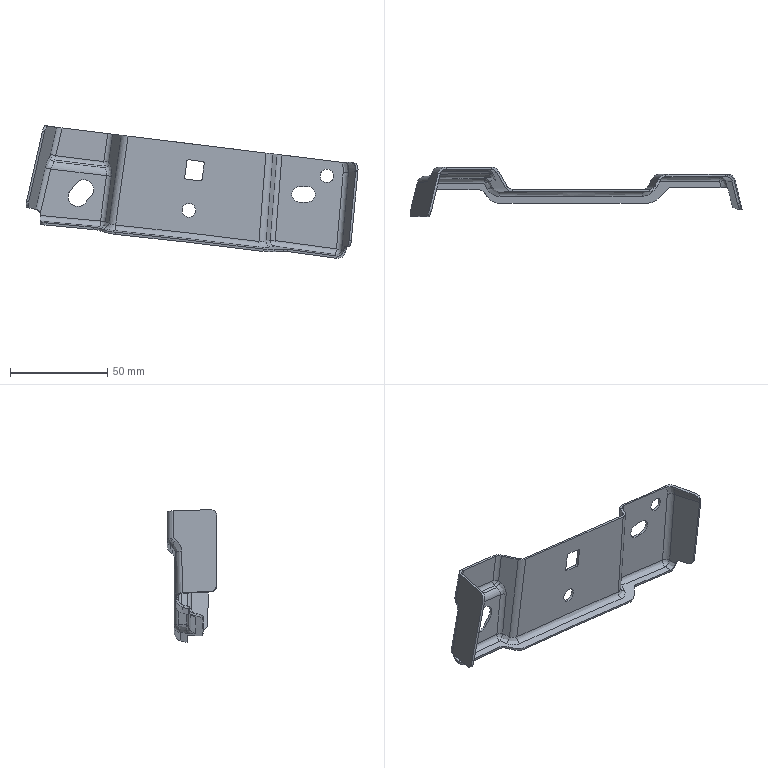Part | STEP file | FNA5401551 | 1 solid | 142 faces | box 170.503 x 25.651 x 68.139 mm | volume 12125 mm3 | spline 63 | cylinder 39 | plane 27 | sphere 10 | other 3 | commonest cylinder face diameters 6 x11 8.4 x10 2 x4 7 x4 8 x4 5.6 x2